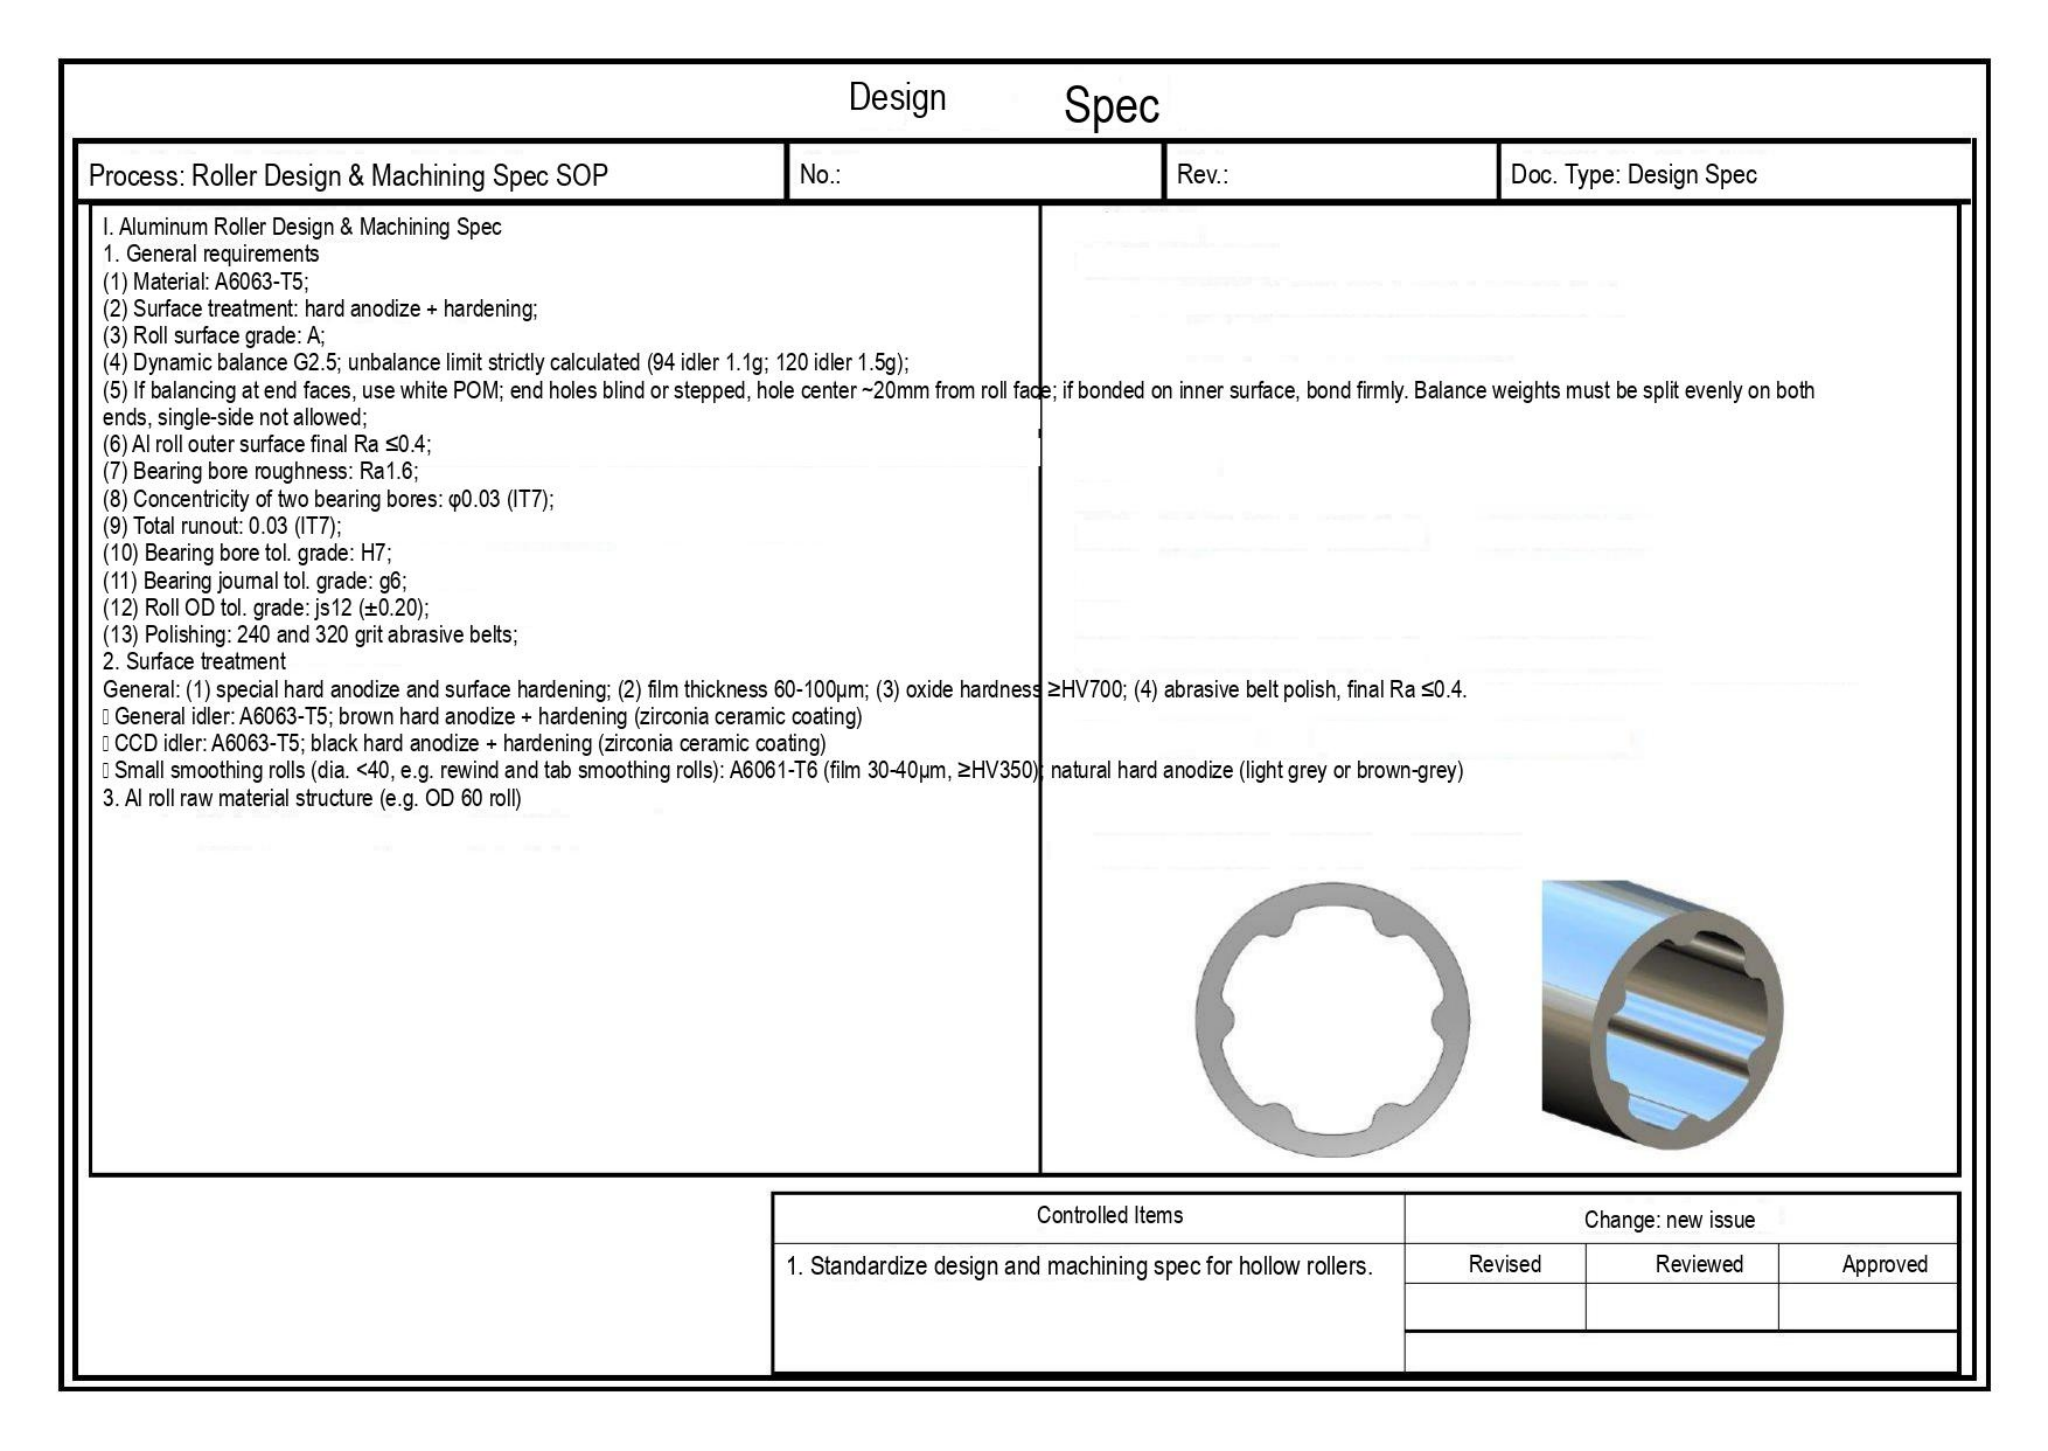Design Spec

| Process: Roller Design & Machining Spec SOP | No.: | Rev.: | Doc. Type: Design Spec |
|---|---|---|---|

I. Aluminum Roller Design & Machining Spec
1. General requirements
(1) Material: A6063-T5;
(2) Surface treatment: hard anodize + hardening;
(3) Roll surface grade: A;
(4) Dynamic balance G2.5; unbalance limit strictly calculated (94 idler 1.1g; 120 idler 1.5g);
(5) If balancing at end faces, use white POM; end holes blind or stepped, hole center ~20mm from roll face; if bonded on inner surface, bond firmly. Balance weights must be split evenly on both ends, single-side not allowed;
(6) Al roll outer surface final Ra ≤0.4;
(7) Bearing bore roughness: Ra1.6;
(8) Concentricity of two bearing bores: φ0.03 (IT7);
(9) Total runout: 0.03 (IT7);
(10) Bearing bore tol. grade: H7;
(11) Bearing journal tol. grade: g6;
(12) Roll OD tol. grade: js12 (±0.20);
(13) Polishing: 240 and 320 grit abrasive belts;
2. Surface treatment
General: (1) special hard anodize and surface hardening; (2) film thickness 60-100μm; (3) oxide hardness ≥HV700; (4) abrasive belt polish, final Ra ≤0.4.
General idler: A6063-T5; brown hard anodize + hardening (zirconia ceramic coating)
CCD idler: A6063-T5; black hard anodize + hardening (zirconia ceramic coating)
Small smoothing rolls (dia. <40, e.g. rewind and tab smoothing rolls): A6061-T6 (film 30-40μm, ≥HV350); natural hard anodize (light grey or brown-grey)
3. Al roll raw material structure (e.g. OD 60 roll)

| Controlled Items | Change: new issue | | |
|---|---|---|---|
| 1. Standardize design and machining spec for hollow rollers. | Revised | Reviewed | Approved |
| | | | |
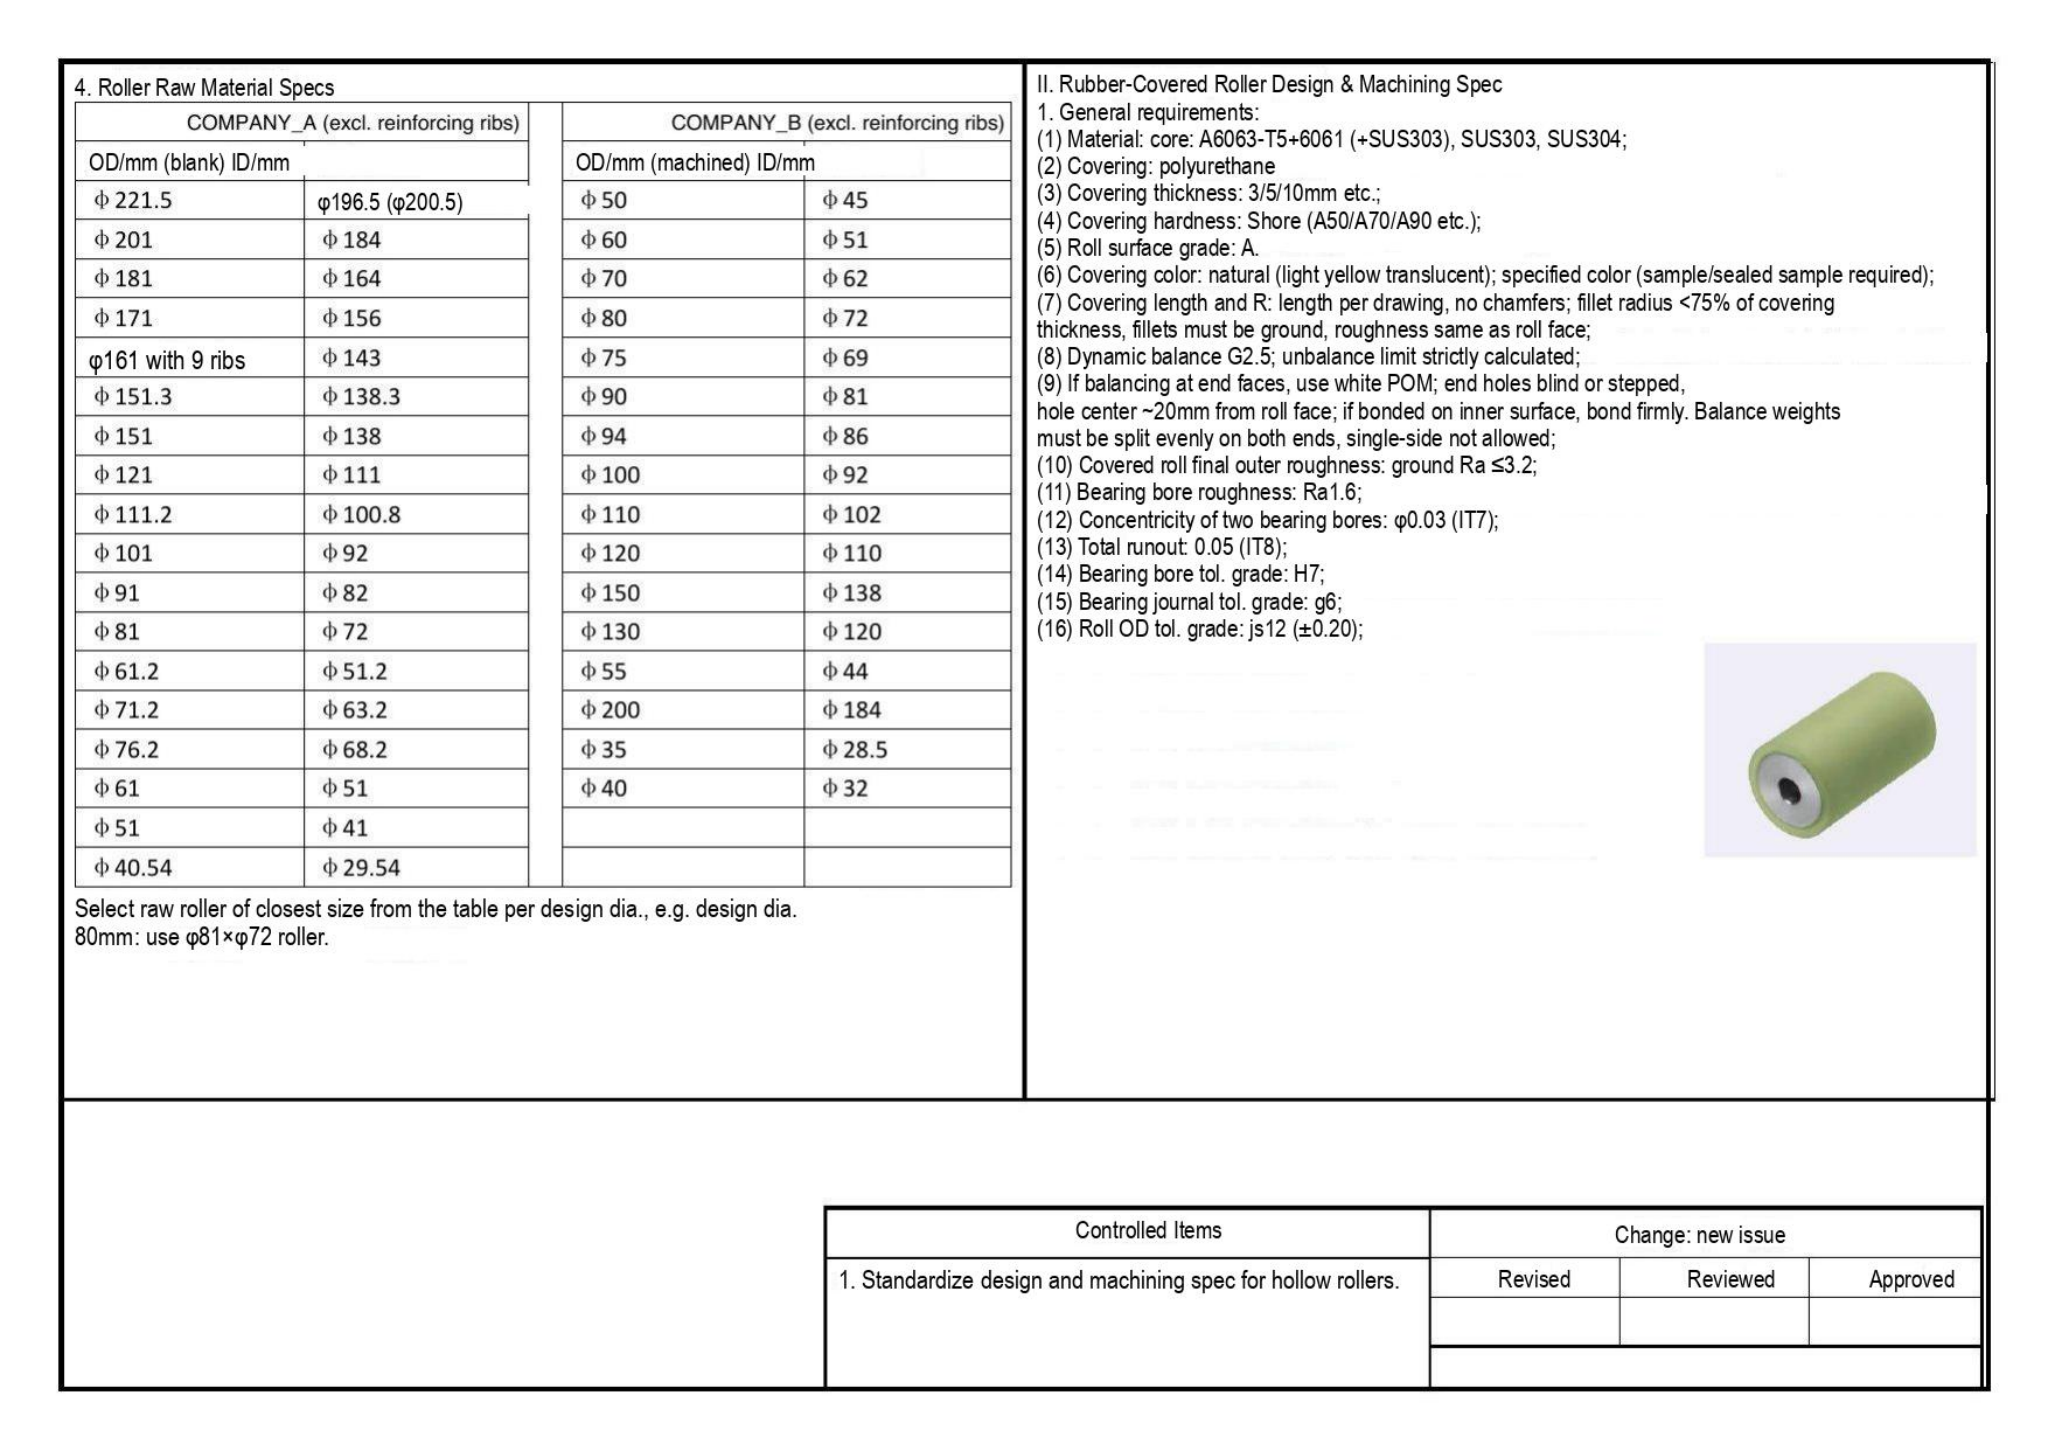4. Roller Raw Material Specs

| COMPANY_A (excl. reinforcing ribs) | | COMPANY_B (excl. reinforcing ribs) | |
|---|---|---|---|
| OD/mm (blank) ID/mm | | OD/mm (machined) ID/mm | |
| ф221.5 | φ196.5 (φ200.5) | ф50 | ф45 |
| ф201 | ф184 | ф60 | ф51 |
| ф181 | ф164 | ф70 | ф62 |
| ф171 | ф156 | ф80 | ф72 |
| φ161 with 9 ribs | ф143 | ф75 | ф69 |
| ф151.3 | ф138.3 | ф90 | ф81 |
| ф151 | ф138 | ф94 | ф86 |
| ф121 | ф111 | ф100 | ф92 |
| ф111.2 | ф100.8 | ф110 | ф102 |
| ф101 | ф92 | ф120 | ф110 |
| ф91 | ф82 | ф150 | ф138 |
| ф81 | ф72 | ф130 | ф120 |
| ф61.2 | ф51.2 | ф55 | ф44 |
| ф71.2 | ф63.2 | ф200 | ф184 |
| ф76.2 | ф68.2 | ф35 | ф28.5 |
| ф61 | ф51 | ф40 | ф32 |
| ф51 | ф41 | | |
| ф40.54 | ф29.54 | | |

Select raw roller of closest size from the table per design dia., e.g. design dia. 80mm: use φ81×φ72 roller.

II. Rubber-Covered Roller Design & Machining Spec
1. General requirements:
(1) Material: core: A6063-T5+6061 (+SUS303), SUS303, SUS304;
(2) Covering: polyurethane
(3) Covering thickness: 3/5/10mm etc.;
(4) Covering hardness: Shore (A50/A70/A90 etc.);
(5) Roll surface grade: A.
(6) Covering color: natural (light yellow translucent); specified color (sample/sealed sample required);
(7) Covering length and R: length per drawing, no chamfers; fillet radius <75% of covering thickness, fillets must be ground, roughness same as roll face;
(8) Dynamic balance G2.5; unbalance limit strictly calculated;
(9) If balancing at end faces, use white POM; end holes blind or stepped, hole center ~20mm from roll face; if bonded on inner surface, bond firmly. Balance weights must be split evenly on both ends, single-side not allowed;
(10) Covered roll final outer roughness: ground Ra ≤3.2;
(11) Bearing bore roughness: Ra1.6;
(12) Concentricity of two bearing bores: φ0.03 (IT7);
(13) Total runout: 0.05 (IT8);
(14) Bearing bore tol. grade: H7;
(15) Bearing journal tol. grade: g6;
(16) Roll OD tol. grade: js12 (±0.20);

| Controlled Items | Change: new issue | | |
|---|---|---|---|
| 1. Standardize design and machining spec for hollow rollers. | Revised | Reviewed | Approved |
| | | | |
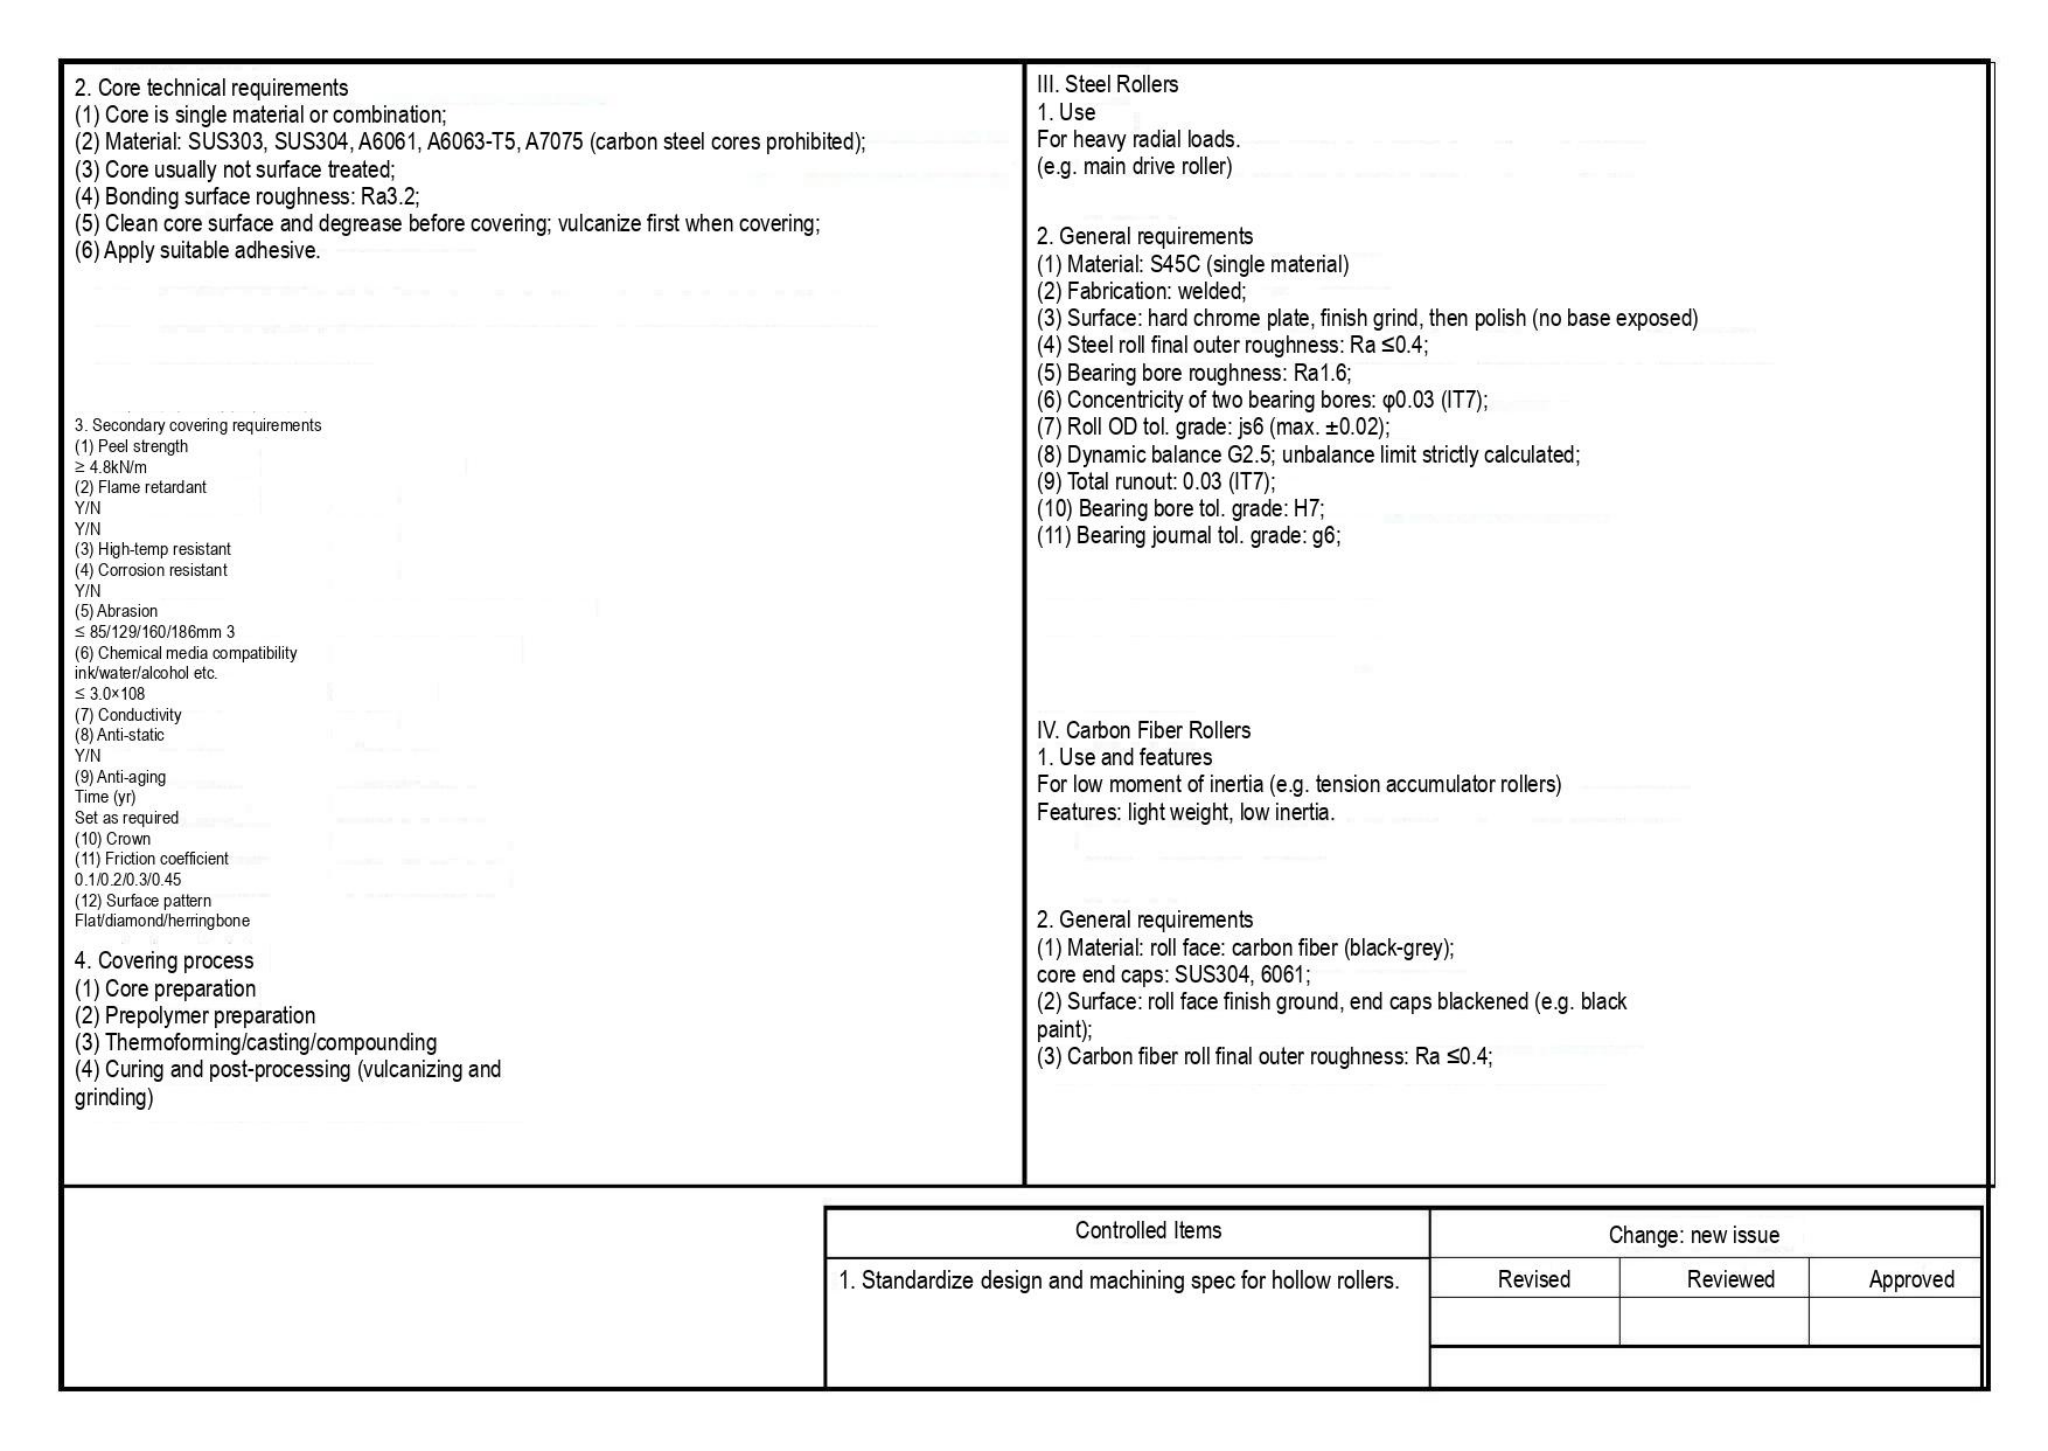2. Core technical requirements
(1) Core is single material or combination;
(2) Material: SUS303, SUS304, A6061, A6063-T5, A7075 (carbon steel cores prohibited);
(3) Core usually not surface treated;
(4) Bonding surface roughness: Ra3.2;
(5) Clean core surface and degrease before covering; vulcanize first when covering;
(6) Apply suitable adhesive.

3. Secondary covering requirements
(1) Peel strength
≥ 4.8kN/m
(2) Flame retardant
Y/N
Y/N
(3) High-temp resistant
(4) Corrosion resistant
Y/N
(5) Abrasion
≤ 85/129/160/186mm 3
(6) Chemical media compatibility
ink/water/alcohol etc.
≤ 3.0×108
(7) Conductivity
(8) Anti-static
Y/N
(9) Anti-aging
Time (yr)
Set as required
(10) Crown
(11) Friction coefficient
0.1/0.2/0.3/0.45
(12) Surface pattern
Flat/diamond/herringbone

4. Covering process
(1) Core preparation
(2) Prepolymer preparation
(3) Thermoforming/casting/compounding
(4) Curing and post-processing (vulcanizing and grinding)

III. Steel Rollers
1. Use
For heavy radial loads.
(e.g. main drive roller)

2. General requirements
(1) Material: S45C (single material)
(2) Fabrication: welded;
(3) Surface: hard chrome plate, finish grind, then polish (no base exposed)
(4) Steel roll final outer roughness: Ra ≤0.4;
(5) Bearing bore roughness: Ra1.6;
(6) Concentricity of two bearing bores: φ0.03 (IT7);
(7) Roll OD tol. grade: js6 (max. ±0.02);
(8) Dynamic balance G2.5; unbalance limit strictly calculated;
(9) Total runout: 0.03 (IT7);
(10) Bearing bore tol. grade: H7;
(11) Bearing journal tol. grade: g6;

IV. Carbon Fiber Rollers
1. Use and features
For low moment of inertia (e.g. tension accumulator rollers)
Features: light weight, low inertia.

2. General requirements
(1) Material: roll face: carbon fiber (black-grey);
core end caps: SUS304, 6061;
(2) Surface: roll face finish ground, end caps blackened (e.g. black paint);
(3) Carbon fiber roll final outer roughness: Ra ≤0.4;

| Controlled Items | Change: new issue | | |
|---|---|---|---|
| 1. Standardize design and machining spec for hollow rollers. | Revised | Reviewed | Approved |
| | | | |
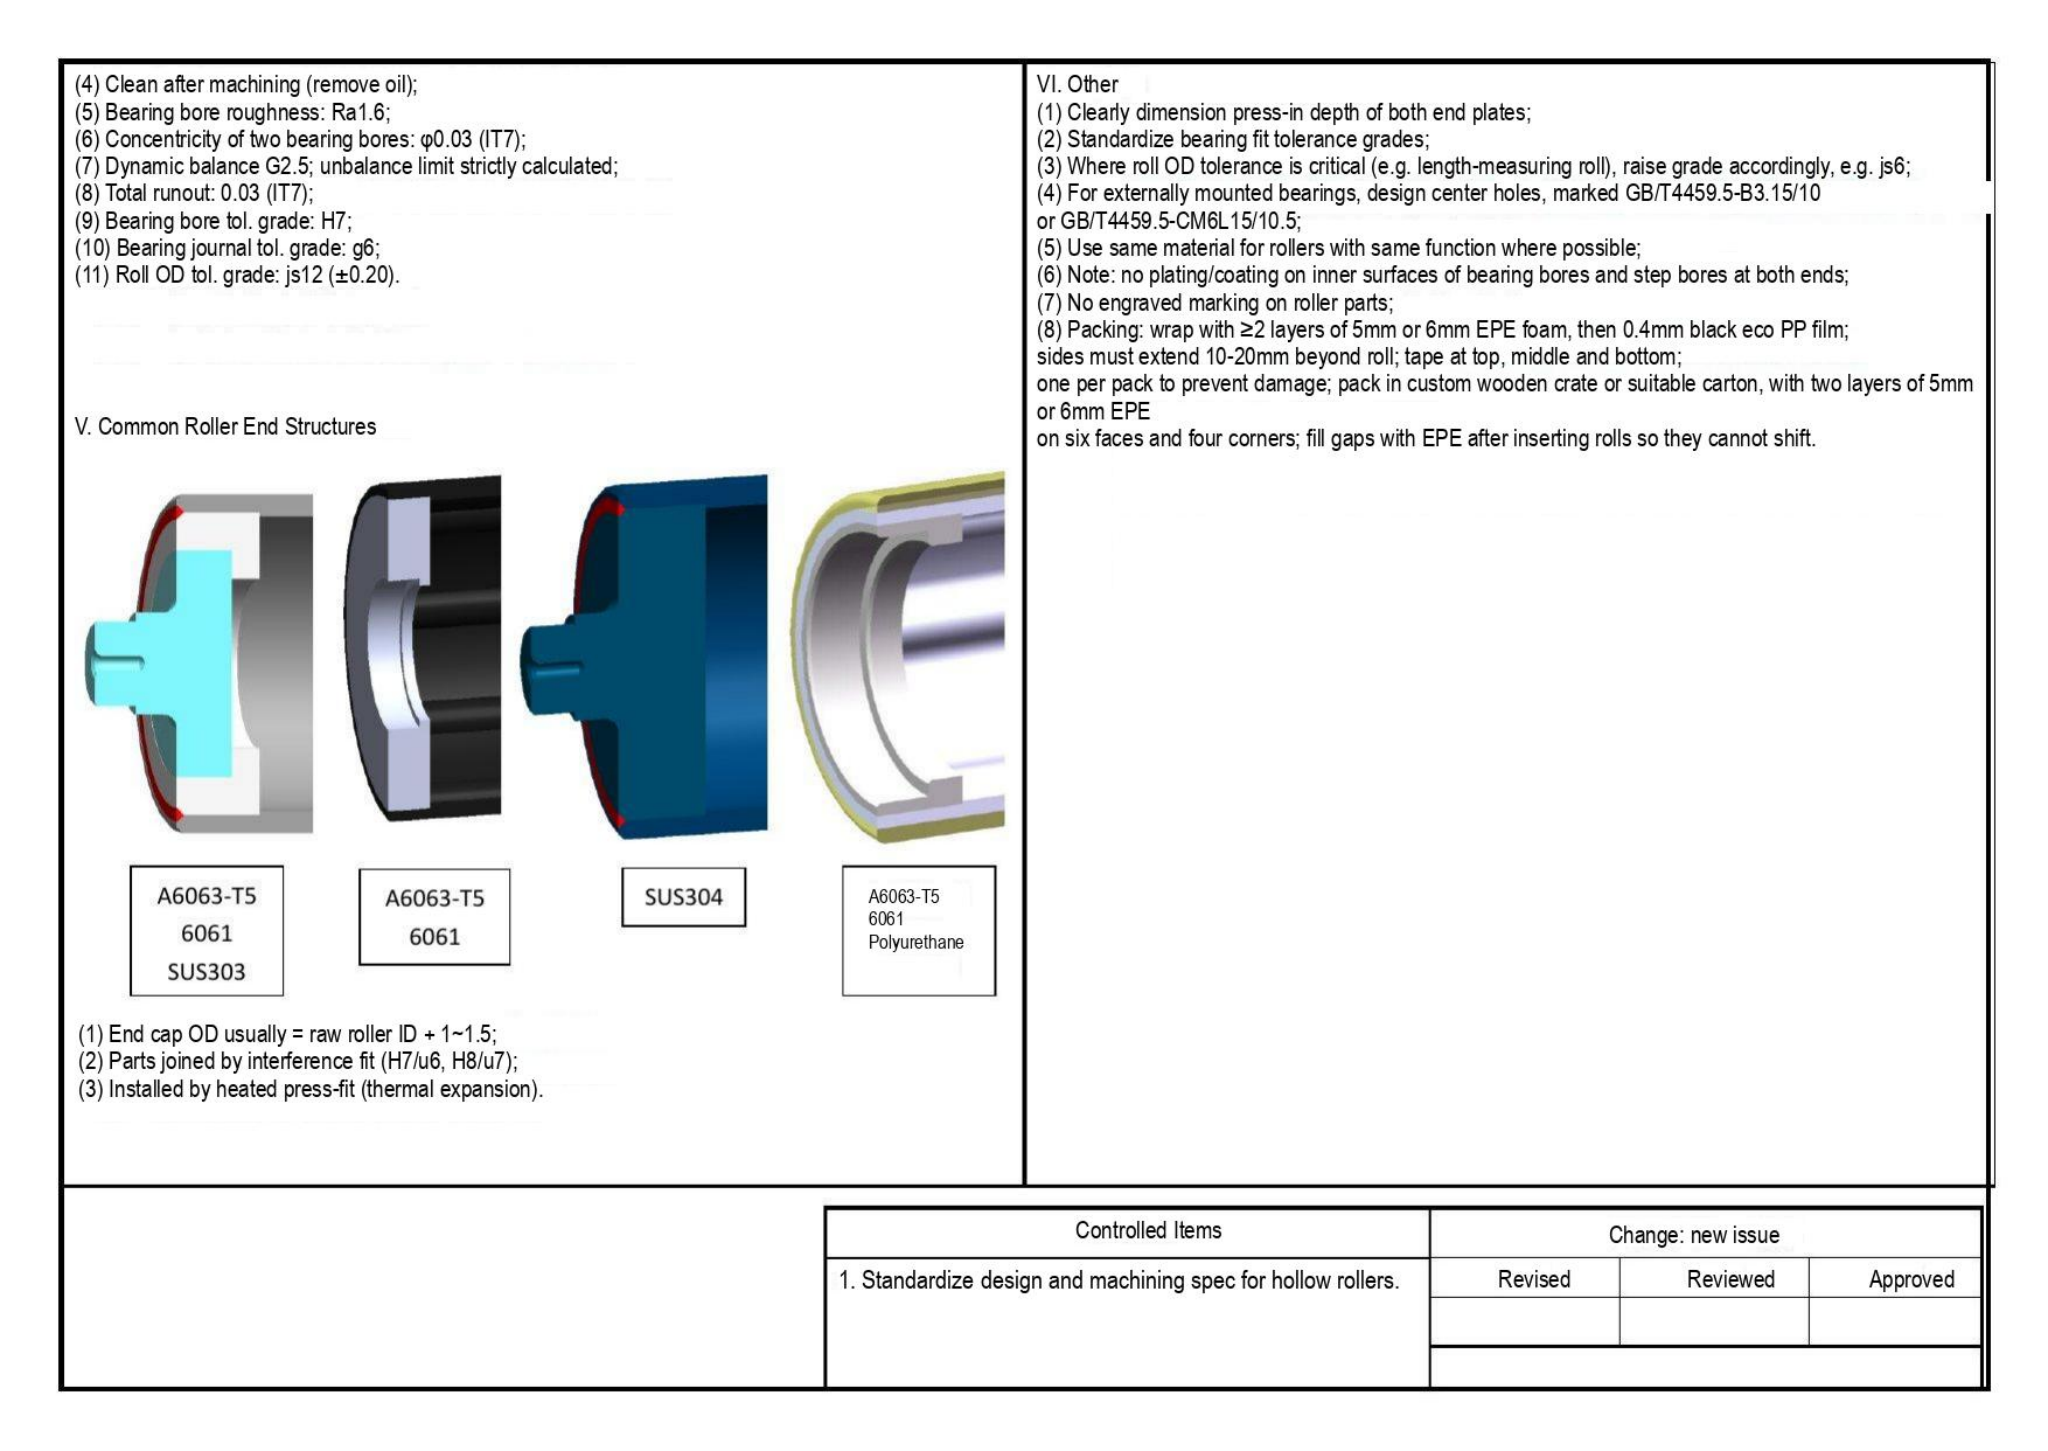(4) Clean after machining (remove oil);
(5) Bearing bore roughness: Ra1.6;
(6) Concentricity of two bearing bores: φ0.03 (IT7);
(7) Dynamic balance G2.5; unbalance limit strictly calculated;
(8) Total runout: 0.03 (IT7);
(9) Bearing bore tol. grade: H7;
(10) Bearing journal tol. grade: g6;
(11) Roll OD tol. grade: js12 (±0.20).

V. Common Roller End Structures

A6063-T5
6061
SUS303

A6063-T5
6061

SUS304

A6063-T5
6061
Polyurethane

(1) End cap OD usually = raw roller ID + 1~1.5;
(2) Parts joined by interference fit (H7/u6, H8/u7);
(3) Installed by heated press-fit (thermal expansion).

VI. Other
(1) Clearly dimension press-in depth of both end plates;
(2) Standardize bearing fit tolerance grades;
(3) Where roll OD tolerance is critical (e.g. length-measuring roll), raise grade accordingly, e.g. js6;
(4) For externally mounted bearings, design center holes, marked GB/T4459.5-B3.15/10
or GB/T4459.5-CM6L15/10.5;
(5) Use same material for rollers with same function where possible;
(6) Note: no plating/coating on inner surfaces of bearing bores and step bores at both ends;
(7) No engraved marking on roller parts;
(8) Packing: wrap with ≥2 layers of 5mm or 6mm EPE foam, then 0.4mm black eco PP film;
sides must extend 10-20mm beyond roll; tape at top, middle and bottom;
one per pack to prevent damage; pack in custom wooden crate or suitable carton, with two layers of 5mm or 6mm EPE
on six faces and four corners; fill gaps with EPE after inserting rolls so they cannot shift.

| Controlled Items | Change: new issue | | |
|---|---|---|---|
| 1. Standardize design and machining spec for hollow rollers. | Revised | Reviewed | Approved |
| | | | |